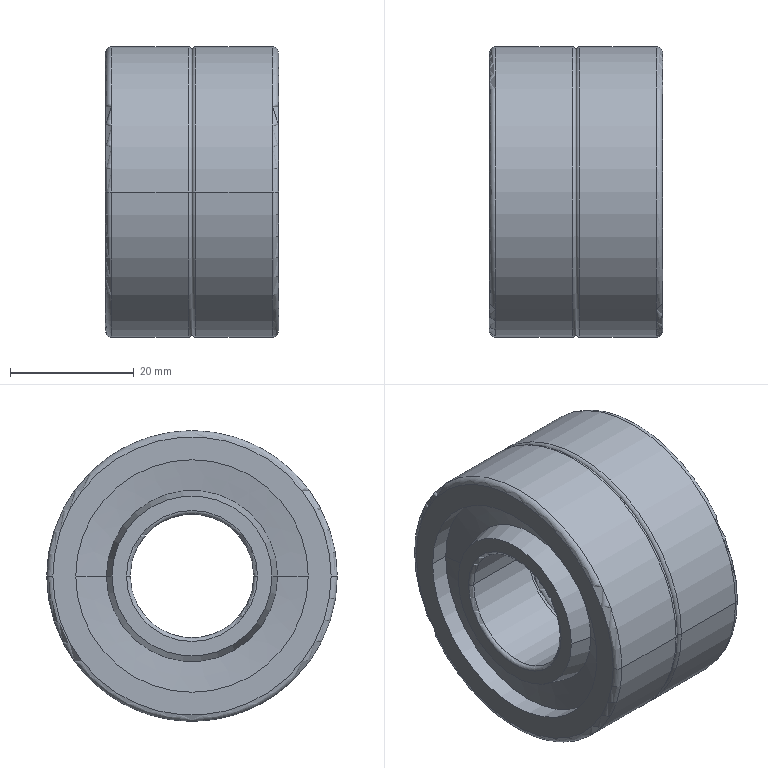Part | NX | 1 solid | 50 faces | box 28 x 47 x 47 mm | volume 32125 mm3 | torus 16 | cone 16 | cylinder 14 | plane 4 | commonest cylinder face diameters 20 x4 37.6 x4 47 x4 29.4 x2
STEP:
#1=CARTESIAN_POINT('',(24.,-11.,0.));
#2=VERTEX_POINT('',#1);
#3=CARTESIAN_POINT('',(23.,-10.,0.));
#4=VERTEX_POINT('',#3);
#5=CARTESIAN_POINT('',(23.,-11.,0.));
#6=DIRECTION('',(0.,0.,-1.));
#7=DIRECTION('',(-1.,0.,0.));
#8=AXIS2_PLACEMENT_3D('',#5,#6,#7);
#9=CIRCLE('',#8,1.);
#10=EDGE_CURVE('',#2,#4,#9,.F.);
#11=ORIENTED_EDGE('',*,*,#10,.T.);
#12=CARTESIAN_POINT('',(23.,10.,0.));
#13=VERTEX_POINT('',#12);
#14=CARTESIAN_POINT('',(23.,0.,0.));
#15=DIRECTION('',(1.,0.,0.));
#16=DIRECTION('',(0.,-1.,0.));
#17=AXIS2_PLACEMENT_3D('',#14,#15,#16);
#18=CIRCLE('',#17,10.);
#19=EDGE_CURVE('',#13,#4,#18,.T.);
#20=ORIENTED_EDGE('',*,*,#19,.F.);
#21=CARTESIAN_POINT('',(24.,11.,0.));
#22=VERTEX_POINT('',#21);
#23=CARTESIAN_POINT('',(23.,11.,0.));
#24=DIRECTION('',(0.,0.,1.));
#25=DIRECTION('',(-1.,0.,0.));
#26=AXIS2_PLACEMENT_3D('',#23,#24,#25);
#27=CIRCLE('',#26,1.);
#28=EDGE_CURVE('',#22,#13,#27,.F.);
#29=ORIENTED_EDGE('',*,*,#28,.F.);
#30=CARTESIAN_POINT('',(24.,0.,0.));
#31=DIRECTION('',(1.,0.,0.));
#32=DIRECTION('',(0.,-1.,0.));
#33=AXIS2_PLACEMENT_3D('',#30,#31,#32);
#34=CIRCLE('',#33,11.);
#35=EDGE_CURVE('',#22,#2,#34,.T.);
#36=ORIENTED_EDGE('',*,*,#35,.T.);
#37=EDGE_LOOP('',(#11,#20,#29,#36));
#38=FACE_BOUND('',#37,.T.);
#39=CARTESIAN_POINT('',(23.,0.,0.));
#40=DIRECTION('',(1.,0.,0.));
#41=DIRECTION('',(0.,-1.,0.));
#42=AXIS2_PLACEMENT_3D('',#39,#40,#41);
#43=TOROIDAL_SURFACE('',#42,11.,1.);
#44=ADVANCED_FACE('',(#38),#43,.T.);
#45=CARTESIAN_POINT('',(38.,-10.6,0.));
#46=VERTEX_POINT('',#45);
#47=CARTESIAN_POINT('',(37.4,-10.,0.));
#48=VERTEX_POINT('',#47);
#49=CARTESIAN_POINT('',(37.4,-10.6,0.));
#50=DIRECTION('',(0.,0.,-1.));
#51=DIRECTION('',(-1.,0.,0.));
#52=AXIS2_PLACEMENT_3D('',#49,#50,#51);
#53=CIRCLE('',#52,0.6);
#54=EDGE_CURVE('',#46,#48,#53,.F.);
#55=ORIENTED_EDGE('',*,*,#54,.T.);
#56=CARTESIAN_POINT('',(37.4,10.,0.));
#57=VERTEX_POINT('',#56);
#58=CARTESIAN_POINT('',(37.4,0.,0.));
#59=DIRECTION('',(1.,0.,0.));
#60=DIRECTION('',(0.,-1.,0.));
#61=AXIS2_PLACEMENT_3D('',#58,#59,#60);
#62=CIRCLE('',#61,10.);
#63=EDGE_CURVE('',#57,#48,#62,.T.);
#64=ORIENTED_EDGE('',*,*,#63,.F.);
#65=CARTESIAN_POINT('',(38.,10.6,0.));
#66=VERTEX_POINT('',#65);
#67=CARTESIAN_POINT('',(37.4,10.6,0.));
#68=DIRECTION('',(0.,0.,1.));
#69=DIRECTION('',(-1.,0.,0.));
#70=AXIS2_PLACEMENT_3D('',#67,#68,#69);
#71=CIRCLE('',#70,0.6);
#72=EDGE_CURVE('',#66,#57,#71,.F.);
#73=ORIENTED_EDGE('',*,*,#72,.F.);
#74=CARTESIAN_POINT('',(38.,0.,0.));
#75=DIRECTION('',(1.,0.,0.));
#76=DIRECTION('',(0.,-1.,0.));
#77=AXIS2_PLACEMENT_3D('',#74,#75,#76);
#78=CIRCLE('',#77,10.6);
#79=EDGE_CURVE('',#66,#46,#78,.T.);
#80=ORIENTED_EDGE('',*,*,#79,.T.);
#81=EDGE_LOOP('',(#55,#64,#73,#80));
#82=FACE_BOUND('',#81,.T.);
#83=CARTESIAN_POINT('',(37.4,0.,0.));
#84=DIRECTION('',(1.,0.,0.));
#85=DIRECTION('',(0.,-1.,0.));
#86=AXIS2_PLACEMENT_3D('',#83,#84,#85);
#87=TOROIDAL_SURFACE('',#86,10.6,0.6);
#88=ADVANCED_FACE('',(#82),#87,.T.);
#89=CARTESIAN_POINT('',(37.,-23.5,0.));
#90=VERTEX_POINT('',#89);
#91=CARTESIAN_POINT('',(37.,23.5,0.));
#92=VERTEX_POINT('',#91);
#93=CARTESIAN_POINT('',(37.,0.,0.));
#94=DIRECTION('',(1.,0.,0.));
#95=DIRECTION('',(0.,-1.,0.));
#96=AXIS2_PLACEMENT_3D('',#93,#94,#95);
#97=CIRCLE('',#96,23.5);
#98=EDGE_CURVE('',#90,#92,#97,.T.);
#99=ORIENTED_EDGE('',*,*,#98,.T.);
#100=CARTESIAN_POINT('',(38.,22.5,0.));
#101=VERTEX_POINT('',#100);
#102=CARTESIAN_POINT('',(37.,22.5,0.));
#103=DIRECTION('',(0.,0.,1.));
#104=DIRECTION('',(-1.,0.,0.));
#105=AXIS2_PLACEMENT_3D('',#102,#103,#104);
#106=CIRCLE('',#105,1.);
#107=EDGE_CURVE('',#101,#92,#106,.T.);
#108=ORIENTED_EDGE('',*,*,#107,.F.);
#109=CARTESIAN_POINT('',(38.,-22.5,0.));
#110=VERTEX_POINT('',#109);
#111=CARTESIAN_POINT('',(38.,0.,0.));
#112=DIRECTION('',(1.,0.,0.));
#113=DIRECTION('',(0.,-1.,0.));
#114=AXIS2_PLACEMENT_3D('',#111,#112,#113);
#115=CIRCLE('',#114,22.5);
#116=EDGE_CURVE('',#110,#101,#115,.T.);
#117=ORIENTED_EDGE('',*,*,#116,.F.);
#118=CARTESIAN_POINT('',(37.,-22.5,0.));
#119=DIRECTION('',(0.,0.,-1.));
#120=DIRECTION('',(-1.,0.,0.));
#121=AXIS2_PLACEMENT_3D('',#118,#119,#120);
#122=CIRCLE('',#121,1.);
#123=EDGE_CURVE('',#110,#90,#122,.T.);
#124=ORIENTED_EDGE('',*,*,#123,.T.);
#125=EDGE_LOOP('',(#99,#108,#117,#124));
#126=FACE_BOUND('',#125,.T.);
#127=CARTESIAN_POINT('',(37.,0.,0.));
#128=DIRECTION('',(1.,0.,0.));
#129=DIRECTION('',(0.,-1.,0.));
#130=AXIS2_PLACEMENT_3D('',#127,#128,#129);
#131=TOROIDAL_SURFACE('',#130,22.5,1.);
#132=ADVANCED_FACE('',(#126),#131,.T.);
#133=CARTESIAN_POINT('',(24.,-22.9,0.));
#134=VERTEX_POINT('',#133);
#135=CARTESIAN_POINT('',(24.,22.9,0.));
#136=VERTEX_POINT('',#135);
#137=CARTESIAN_POINT('',(24.,0.,0.));
#138=DIRECTION('',(1.,0.,0.));
#139=DIRECTION('',(0.,-1.,0.));
#140=AXIS2_PLACEMENT_3D('',#137,#138,#139);
#141=CIRCLE('',#140,22.9);
#142=EDGE_CURVE('',#134,#136,#141,.T.);
#143=ORIENTED_EDGE('',*,*,#142,.F.);
#144=CARTESIAN_POINT('',(23.4,-23.5,0.));
#145=VERTEX_POINT('',#144);
#146=CARTESIAN_POINT('',(23.4,-22.9,0.));
#147=DIRECTION('',(0.,0.,-1.));
#148=DIRECTION('',(-1.,0.,0.));
#149=AXIS2_PLACEMENT_3D('',#146,#147,#148);
#150=CIRCLE('',#149,0.6);
#151=EDGE_CURVE('',#145,#134,#150,.F.);
#152=ORIENTED_EDGE('',*,*,#151,.F.);
#153=CARTESIAN_POINT('',(23.4,23.5,0.));
#154=VERTEX_POINT('',#153);
#155=CARTESIAN_POINT('',(23.4,0.,0.));
#156=DIRECTION('',(1.,0.,0.));
#157=DIRECTION('',(0.,-1.,0.));
#158=AXIS2_PLACEMENT_3D('',#155,#156,#157);
#159=CIRCLE('',#158,23.5);
#160=EDGE_CURVE('',#145,#154,#159,.T.);
#161=ORIENTED_EDGE('',*,*,#160,.T.);
#162=CARTESIAN_POINT('',(23.4,22.9,0.));
#163=DIRECTION('',(0.,0.,1.));
#164=DIRECTION('',(-1.,0.,0.));
#165=AXIS2_PLACEMENT_3D('',#162,#163,#164);
#166=CIRCLE('',#165,0.6);
#167=EDGE_CURVE('',#154,#136,#166,.F.);
#168=ORIENTED_EDGE('',*,*,#167,.T.);
#169=EDGE_LOOP('',(#143,#152,#161,#168));
#170=FACE_BOUND('',#169,.T.);
#171=CARTESIAN_POINT('',(23.4,0.,0.));
#172=DIRECTION('',(1.,0.,0.));
#173=DIRECTION('',(0.,-1.,0.));
#174=AXIS2_PLACEMENT_3D('',#171,#172,#173);
#175=TOROIDAL_SURFACE('',#174,22.9,0.6);
#176=ADVANCED_FACE('',(#170),#175,.T.);
#177=CARTESIAN_POINT('',(24.6,23.5,0.));
#178=VERTEX_POINT('',#177);
#179=CARTESIAN_POINT('',(24.6,-23.5,0.));
#180=VERTEX_POINT('',#179);
#181=CARTESIAN_POINT('',(24.6,0.,0.));
#182=DIRECTION('',(1.,0.,0.));
#183=DIRECTION('',(0.,-1.,0.));
#184=AXIS2_PLACEMENT_3D('',#181,#182,#183);
#185=CIRCLE('',#184,23.5);
#186=EDGE_CURVE('',#178,#180,#185,.T.);
#187=ORIENTED_EDGE('',*,*,#186,.F.);
#188=CARTESIAN_POINT('',(24.6,22.9,0.));
#189=DIRECTION('',(0.,0.,1.));
#190=DIRECTION('',(-1.,0.,0.));
#191=AXIS2_PLACEMENT_3D('',#188,#189,#190);
#192=CIRCLE('',#191,0.6);
#193=EDGE_CURVE('',#178,#136,#192,.T.);
#194=ORIENTED_EDGE('',*,*,#193,.T.);
#195=CARTESIAN_POINT('',(24.,0.,0.));
#196=DIRECTION('',(1.,0.,0.));
#197=DIRECTION('',(0.,-1.,0.));
#198=AXIS2_PLACEMENT_3D('',#195,#196,#197);
#199=CIRCLE('',#198,22.9);
#200=EDGE_CURVE('',#136,#134,#199,.T.);
#201=ORIENTED_EDGE('',*,*,#200,.T.);
#202=CARTESIAN_POINT('',(24.6,-22.9,0.));
#203=DIRECTION('',(0.,0.,-1.));
#204=DIRECTION('',(-1.,0.,0.));
#205=AXIS2_PLACEMENT_3D('',#202,#203,#204);
#206=CIRCLE('',#205,0.6);
#207=EDGE_CURVE('',#180,#134,#206,.T.);
#208=ORIENTED_EDGE('',*,*,#207,.F.);
#209=EDGE_LOOP('',(#187,#194,#201,#208));
#210=FACE_BOUND('',#209,.T.);
#211=CARTESIAN_POINT('',(24.6,0.,0.));
#212=DIRECTION('',(1.,0.,0.));
#213=DIRECTION('',(0.,-1.,0.));
#214=AXIS2_PLACEMENT_3D('',#211,#212,#213);
#215=TOROIDAL_SURFACE('',#214,22.9,0.6);
#216=ADVANCED_FACE('',(#210),#215,.T.);
#217=CARTESIAN_POINT('',(10.,22.5,0.));
#218=VERTEX_POINT('',#217);
#219=CARTESIAN_POINT('',(10.,-22.5,0.));
#220=VERTEX_POINT('',#219);
#221=CARTESIAN_POINT('',(10.,0.,0.));
#222=DIRECTION('',(1.,0.,0.));
#223=DIRECTION('',(0.,-1.,0.));
#224=AXIS2_PLACEMENT_3D('',#221,#222,#223);
#225=CIRCLE('',#224,22.5);
#226=EDGE_CURVE('',#218,#220,#225,.T.);
#227=ORIENTED_EDGE('',*,*,#226,.T.);
#228=CARTESIAN_POINT('',(11.,-23.5,0.));
#229=VERTEX_POINT('',#228);
#230=CARTESIAN_POINT('',(11.,-22.5,0.));
#231=DIRECTION('',(0.,0.,-1.));
#232=DIRECTION('',(-1.,0.,0.));
#233=AXIS2_PLACEMENT_3D('',#230,#231,#232);
#234=CIRCLE('',#233,1.);
#235=EDGE_CURVE('',#220,#229,#234,.F.);
#236=ORIENTED_EDGE('',*,*,#235,.T.);
#237=CARTESIAN_POINT('',(11.,23.5,0.));
#238=VERTEX_POINT('',#237);
#239=CARTESIAN_POINT('',(11.,0.,0.));
#240=DIRECTION('',(1.,0.,0.));
#241=DIRECTION('',(0.,-1.,0.));
#242=AXIS2_PLACEMENT_3D('',#239,#240,#241);
#243=CIRCLE('',#242,23.5);
#244=EDGE_CURVE('',#238,#229,#243,.T.);
#245=ORIENTED_EDGE('',*,*,#244,.F.);
#246=CARTESIAN_POINT('',(11.,22.5,0.));
#247=DIRECTION('',(0.,0.,1.));
#248=DIRECTION('',(-1.,0.,0.));
#249=AXIS2_PLACEMENT_3D('',#246,#247,#248);
#250=CIRCLE('',#249,1.);
#251=EDGE_CURVE('',#218,#238,#250,.F.);
#252=ORIENTED_EDGE('',*,*,#251,.F.);
#253=EDGE_LOOP('',(#227,#236,#245,#252));
#254=FACE_BOUND('',#253,.T.);
#255=CARTESIAN_POINT('',(11.,0.,0.));
#256=DIRECTION('',(1.,0.,0.));
#257=DIRECTION('',(0.,-1.,0.));
#258=AXIS2_PLACEMENT_3D('',#255,#256,#257);
#259=TOROIDAL_SURFACE('',#258,22.5,1.);
#260=ADVANCED_FACE('',(#254),#259,.T.);
#261=CARTESIAN_POINT('',(10.,-10.6,0.));
#262=VERTEX_POINT('',#261);
#263=CARTESIAN_POINT('',(10.,10.6,0.));
#264=VERTEX_POINT('',#263);
#265=CARTESIAN_POINT('',(10.,0.,0.));
#266=DIRECTION('',(1.,0.,0.));
#267=DIRECTION('',(0.,-1.,0.));
#268=AXIS2_PLACEMENT_3D('',#265,#266,#267);
#269=CIRCLE('',#268,10.6);
#270=EDGE_CURVE('',#262,#264,#269,.T.);
#271=ORIENTED_EDGE('',*,*,#270,.F.);
#272=CARTESIAN_POINT('',(10.6,-10.,0.));
#273=VERTEX_POINT('',#272);
#274=CARTESIAN_POINT('',(10.6,-10.6,0.));
#275=DIRECTION('',(0.,0.,-1.));
#276=DIRECTION('',(-1.,0.,0.));
#277=AXIS2_PLACEMENT_3D('',#274,#275,#276);
#278=CIRCLE('',#277,0.6);
#279=EDGE_CURVE('',#273,#262,#278,.F.);
#280=ORIENTED_EDGE('',*,*,#279,.F.);
#281=CARTESIAN_POINT('',(10.6,10.,0.));
#282=VERTEX_POINT('',#281);
#283=CARTESIAN_POINT('',(10.6,0.,0.));
#284=DIRECTION('',(1.,0.,0.));
#285=DIRECTION('',(0.,-1.,0.));
#286=AXIS2_PLACEMENT_3D('',#283,#284,#285);
#287=CIRCLE('',#286,10.);
#288=EDGE_CURVE('',#273,#282,#287,.T.);
#289=ORIENTED_EDGE('',*,*,#288,.T.);
#290=CARTESIAN_POINT('',(10.6,10.6,0.));
#291=DIRECTION('',(0.,0.,1.));
#292=DIRECTION('',(-1.,0.,0.));
#293=AXIS2_PLACEMENT_3D('',#290,#291,#292);
#294=CIRCLE('',#293,0.6);
#295=EDGE_CURVE('',#282,#264,#294,.F.);
#296=ORIENTED_EDGE('',*,*,#295,.T.);
#297=EDGE_LOOP('',(#271,#280,#289,#296));
#298=FACE_BOUND('',#297,.T.);
#299=CARTESIAN_POINT('',(10.6,0.,0.));
#300=DIRECTION('',(1.,0.,0.));
#301=DIRECTION('',(0.,-1.,0.));
#302=AXIS2_PLACEMENT_3D('',#299,#300,#301);
#303=TOROIDAL_SURFACE('',#302,10.6,0.6);
#304=ADVANCED_FACE('',(#298),#303,.T.);
#305=CARTESIAN_POINT('',(25.,10.,0.));
#306=VERTEX_POINT('',#305);
#307=CARTESIAN_POINT('',(25.,-10.,0.));
#308=VERTEX_POINT('',#307);
#309=CARTESIAN_POINT('',(25.,0.,0.));
#310=DIRECTION('',(1.,0.,0.));
#311=DIRECTION('',(0.,-1.,0.));
#312=AXIS2_PLACEMENT_3D('',#309,#310,#311);
#313=CIRCLE('',#312,10.);
#314=EDGE_CURVE('',#306,#308,#313,.T.);
#315=ORIENTED_EDGE('',*,*,#314,.T.);
#316=CARTESIAN_POINT('',(25.,-11.,0.));
#317=DIRECTION('',(0.,0.,-1.));
#318=DIRECTION('',(-1.,0.,0.));
#319=AXIS2_PLACEMENT_3D('',#316,#317,#318);
#320=CIRCLE('',#319,1.);
#321=EDGE_CURVE('',#308,#2,#320,.F.);
#322=ORIENTED_EDGE('',*,*,#321,.T.);
#323=ORIENTED_EDGE('',*,*,#35,.F.);
#324=CARTESIAN_POINT('',(25.,11.,0.));
#325=DIRECTION('',(0.,0.,1.));
#326=DIRECTION('',(-1.,0.,0.));
#327=AXIS2_PLACEMENT_3D('',#324,#325,#326);
#328=CIRCLE('',#327,1.);
#329=EDGE_CURVE('',#306,#22,#328,.F.);
#330=ORIENTED_EDGE('',*,*,#329,.F.);
#331=EDGE_LOOP('',(#315,#322,#323,#330));
#332=FACE_BOUND('',#331,.T.);
#333=CARTESIAN_POINT('',(25.,0.,0.));
#334=DIRECTION('',(1.,0.,0.));
#335=DIRECTION('',(0.,-1.,0.));
#336=AXIS2_PLACEMENT_3D('',#333,#334,#335);
#337=TOROIDAL_SURFACE('',#336,11.,1.);
#338=ADVANCED_FACE('',(#332),#337,.T.);
#339=CARTESIAN_POINT('',(34.43,13.836,0.));
#340=VERTEX_POINT('',#339);
#341=CARTESIAN_POINT('',(34.43,-13.836,0.));
#342=VERTEX_POINT('',#341);
#343=CARTESIAN_POINT('',(34.43,0.,0.));
#344=DIRECTION('',(1.,0.,0.));
#345=DIRECTION('',(0.,-1.,0.));
#346=AXIS2_PLACEMENT_3D('',#343,#344,#345);
#347=CIRCLE('',#346,13.836);
#348=EDGE_CURVE('',#340,#342,#347,.T.);
#349=ORIENTED_EDGE('',*,*,#348,.F.);
#350=CARTESIAN_POINT('',(35.006,18.8,0.));
#351=VERTEX_POINT('',#350);
#352=CARTESIAN_POINT('',(34.718,16.318,0.));
#353=DIRECTION('',(0.1154,0.9933,0.));
#354=VECTOR('',#353,1000.);
#355=LINE('',#352,#354);
#356=EDGE_CURVE('',#340,#351,#355,.T.);
#357=ORIENTED_EDGE('',*,*,#356,.T.);
#358=CARTESIAN_POINT('',(35.006,-18.8,0.));
#359=VERTEX_POINT('',#358);
#360=CARTESIAN_POINT('',(35.006,0.,0.));
#361=DIRECTION('',(1.,0.,0.));
#362=DIRECTION('',(0.,-1.,0.));
#363=AXIS2_PLACEMENT_3D('',#360,#361,#362);
#364=CIRCLE('',#363,18.8);
#365=EDGE_CURVE('',#351,#359,#364,.T.);
#366=ORIENTED_EDGE('',*,*,#365,.T.);
#367=CARTESIAN_POINT('',(34.718,-16.318,0.));
#368=DIRECTION('',(0.1154,-0.9933,0.));
#369=VECTOR('',#368,1000.);
#370=LINE('',#367,#369);
#371=EDGE_CURVE('',#342,#359,#370,.T.);
#372=ORIENTED_EDGE('',*,*,#371,.F.);
#373=EDGE_LOOP('',(#349,#357,#366,#372));
#374=FACE_BOUND('',#373,.T.);
#375=CARTESIAN_POINT('',(34.718,0.,0.));
#376=DIRECTION('',(1.,0.,0.));
#377=DIRECTION('',(0.,-1.,0.));
#378=AXIS2_PLACEMENT_3D('',#375,#376,#377);
#379=CONICAL_SURFACE('',#378,16.318,1.455);
#380=ADVANCED_FACE('',(#374),#379,.F.);
#381=CARTESIAN_POINT('',(13.57,-13.836,0.));
#382=VERTEX_POINT('',#381);
#383=CARTESIAN_POINT('',(10.,-12.938,0.));
#384=VERTEX_POINT('',#383);
#385=CARTESIAN_POINT('',(11.785,-13.387,0.));
#386=DIRECTION('',(0.9697,-0.2442,0.));
#387=VECTOR('',#386,1000.);
#388=LINE('',#385,#387);
#389=EDGE_CURVE('',#382,#384,#388,.F.);
#390=ORIENTED_EDGE('',*,*,#389,.T.);
#391=CARTESIAN_POINT('',(10.,12.938,0.));
#392=VERTEX_POINT('',#391);
#393=CARTESIAN_POINT('',(10.,0.,0.));
#394=DIRECTION('',(1.,0.,0.));
#395=DIRECTION('',(0.,-1.,0.));
#396=AXIS2_PLACEMENT_3D('',#393,#394,#395);
#397=CIRCLE('',#396,12.938);
#398=EDGE_CURVE('',#384,#392,#397,.T.);
#399=ORIENTED_EDGE('',*,*,#398,.T.);
#400=CARTESIAN_POINT('',(13.57,13.836,0.));
#401=VERTEX_POINT('',#400);
#402=CARTESIAN_POINT('',(11.785,13.387,0.));
#403=DIRECTION('',(0.9697,0.2442,0.));
#404=VECTOR('',#403,1000.);
#405=LINE('',#402,#404);
#406=EDGE_CURVE('',#401,#392,#405,.F.);
#407=ORIENTED_EDGE('',*,*,#406,.F.);
#408=CARTESIAN_POINT('',(13.57,0.,0.));
#409=DIRECTION('',(1.,0.,0.));
#410=DIRECTION('',(0.,-1.,0.));
#411=AXIS2_PLACEMENT_3D('',#408,#409,#410);
#412=CIRCLE('',#411,13.836);
#413=EDGE_CURVE('',#382,#401,#412,.T.);
#414=ORIENTED_EDGE('',*,*,#413,.F.);
#415=EDGE_LOOP('',(#390,#399,#407,#414));
#416=FACE_BOUND('',#415,.T.);
#417=CARTESIAN_POINT('',(11.785,0.,0.));
#418=DIRECTION('',(1.,0.,0.));
#419=DIRECTION('',(0.,-1.,0.));
#420=AXIS2_PLACEMENT_3D('',#417,#418,#419);
#421=CONICAL_SURFACE('',#420,13.387,0.2467);
#422=ADVANCED_FACE('',(#416),#421,.T.);
#423=CARTESIAN_POINT('',(10.6,0.,0.));
#424=DIRECTION('',(1.,0.,0.));
#425=DIRECTION('',(0.,-1.,0.));
#426=AXIS2_PLACEMENT_3D('',#423,#424,#425);
#427=CIRCLE('',#426,10.);
#428=EDGE_CURVE('',#282,#273,#427,.T.);
#429=ORIENTED_EDGE('',*,*,#428,.F.);
#430=CARTESIAN_POINT('',(16.8,10.,0.));
#431=DIRECTION('',(-1.,0.,0.));
#432=VECTOR('',#431,1000.);
#433=LINE('',#430,#432);
#434=EDGE_CURVE('',#13,#282,#433,.T.);
#435=ORIENTED_EDGE('',*,*,#434,.F.);
#436=ORIENTED_EDGE('',*,*,#19,.T.);
#437=CARTESIAN_POINT('',(16.8,-10.,0.));
#438=DIRECTION('',(-1.,0.,0.));
#439=VECTOR('',#438,1000.);
#440=LINE('',#437,#439);
#441=EDGE_CURVE('',#4,#273,#440,.T.);
#442=ORIENTED_EDGE('',*,*,#441,.T.);
#443=EDGE_LOOP('',(#429,#435,#436,#442));
#444=FACE_BOUND('',#443,.T.);
#445=CARTESIAN_POINT('',(16.8,0.,0.));
#446=DIRECTION('',(-1.,0.,0.));
#447=DIRECTION('',(0.,-1.,0.));
#448=AXIS2_PLACEMENT_3D('',#445,#446,#447);
#449=CYLINDRICAL_SURFACE('',#448,10.);
#450=ADVANCED_FACE('',(#444),#449,.F.);
#451=ORIENTED_EDGE('',*,*,#314,.F.);
#452=CARTESIAN_POINT('',(31.2,10.,0.));
#453=DIRECTION('',(-1.,0.,0.));
#454=VECTOR('',#453,1000.);
#455=LINE('',#452,#454);
#456=EDGE_CURVE('',#57,#306,#455,.T.);
#457=ORIENTED_EDGE('',*,*,#456,.F.);
#458=ORIENTED_EDGE('',*,*,#63,.T.);
#459=CARTESIAN_POINT('',(31.2,-10.,0.));
#460=DIRECTION('',(-1.,0.,0.));
#461=VECTOR('',#460,1000.);
#462=LINE('',#459,#461);
#463=EDGE_CURVE('',#48,#308,#462,.T.);
#464=ORIENTED_EDGE('',*,*,#463,.T.);
#465=EDGE_LOOP('',(#451,#457,#458,#464));
#466=FACE_BOUND('',#465,.T.);
#467=CARTESIAN_POINT('',(31.2,0.,0.));
#468=DIRECTION('',(-1.,0.,0.));
#469=DIRECTION('',(0.,-1.,0.));
#470=AXIS2_PLACEMENT_3D('',#467,#468,#469);
#471=CYLINDRICAL_SURFACE('',#470,10.);
#472=ADVANCED_FACE('',(#466),#471,.F.);
#473=CARTESIAN_POINT('',(38.,12.938,0.));
#474=VERTEX_POINT('',#473);
#475=CARTESIAN_POINT('',(36.215,13.387,0.));
#476=DIRECTION('',(-0.9697,0.2442,0.));
#477=VECTOR('',#476,1000.);
#478=LINE('',#475,#477);
#479=EDGE_CURVE('',#474,#340,#478,.T.);
#480=ORIENTED_EDGE('',*,*,#479,.F.);
#481=CARTESIAN_POINT('',(38.,-12.938,0.));
#482=VERTEX_POINT('',#481);
#483=CARTESIAN_POINT('',(38.,0.,0.));
#484=DIRECTION('',(1.,0.,0.));
#485=DIRECTION('',(0.,-1.,0.));
#486=AXIS2_PLACEMENT_3D('',#483,#484,#485);
#487=CIRCLE('',#486,12.938);
#488=EDGE_CURVE('',#482,#474,#487,.T.);
#489=ORIENTED_EDGE('',*,*,#488,.F.);
#490=CARTESIAN_POINT('',(36.215,-13.387,0.));
#491=DIRECTION('',(-0.9697,-0.2442,0.));
#492=VECTOR('',#491,1000.);
#493=LINE('',#490,#492);
#494=EDGE_CURVE('',#482,#342,#493,.T.);
#495=ORIENTED_EDGE('',*,*,#494,.T.);
#496=CARTESIAN_POINT('',(34.43,0.,0.));
#497=DIRECTION('',(1.,0.,0.));
#498=DIRECTION('',(0.,-1.,0.));
#499=AXIS2_PLACEMENT_3D('',#496,#497,#498);
#500=CIRCLE('',#499,13.836);
#501=EDGE_CURVE('',#342,#340,#500,.T.);
#502=ORIENTED_EDGE('',*,*,#501,.T.);
#503=EDGE_LOOP('',(#480,#489,#495,#502));
#504=FACE_BOUND('',#503,.T.);
#505=CARTESIAN_POINT('',(36.215,0.,0.));
#506=DIRECTION('',(-1.,0.,0.));
#507=DIRECTION('',(0.,1.,0.));
#508=AXIS2_PLACEMENT_3D('',#505,#506,#507);
#509=CONICAL_SURFACE('',#508,13.387,0.2467);
#510=ADVANCED_FACE('',(#504),#509,.T.);
#511=CARTESIAN_POINT('',(12.994,-18.8,0.));
#512=VERTEX_POINT('',#511);
#513=CARTESIAN_POINT('',(12.994,18.8,0.));
#514=VERTEX_POINT('',#513);
#515=CARTESIAN_POINT('',(12.994,0.,0.));
#516=DIRECTION('',(1.,0.,0.));
#517=DIRECTION('',(0.,-1.,0.));
#518=AXIS2_PLACEMENT_3D('',#515,#516,#517);
#519=CIRCLE('',#518,18.8);
#520=EDGE_CURVE('',#512,#514,#519,.T.);
#521=ORIENTED_EDGE('',*,*,#520,.F.);
#522=CARTESIAN_POINT('',(13.282,-16.318,0.));
#523=DIRECTION('',(-0.1154,-0.9933,0.));
#524=VECTOR('',#523,1000.);
#525=LINE('',#522,#524);
#526=EDGE_CURVE('',#512,#382,#525,.F.);
#527=ORIENTED_EDGE('',*,*,#526,.T.);
#528=ORIENTED_EDGE('',*,*,#413,.T.);
#529=CARTESIAN_POINT('',(13.282,16.318,0.));
#530=DIRECTION('',(-0.1154,0.9933,0.));
#531=VECTOR('',#530,1000.);
#532=LINE('',#529,#531);
#533=EDGE_CURVE('',#514,#401,#532,.F.);
#534=ORIENTED_EDGE('',*,*,#533,.F.);
#535=EDGE_LOOP('',(#521,#527,#528,#534));
#536=FACE_BOUND('',#535,.T.);
#537=CARTESIAN_POINT('',(13.282,0.,0.));
#538=DIRECTION('',(-1.,0.,0.));
#539=DIRECTION('',(0.,1.,0.));
#540=AXIS2_PLACEMENT_3D('',#537,#538,#539);
#541=CONICAL_SURFACE('',#540,16.318,1.455);
#542=ADVANCED_FACE('',(#536),#541,.F.);
#543=CARTESIAN_POINT('',(38.,-18.8,0.));
#544=VERTEX_POINT('',#543);
#545=CARTESIAN_POINT('',(36.503,-18.8,0.));
#546=DIRECTION('',(-1.,0.,0.));
#547=VECTOR('',#546,1000.);
#548=LINE('',#545,#547);
#549=EDGE_CURVE('',#544,#359,#548,.T.);
#550=ORIENTED_EDGE('',*,*,#549,.T.);
#551=ORIENTED_EDGE('',*,*,#365,.F.);
#552=CARTESIAN_POINT('',(38.,18.8,0.));
#553=VERTEX_POINT('',#552);
#554=CARTESIAN_POINT('',(36.503,18.8,0.));
#555=DIRECTION('',(-1.,0.,0.));
#556=VECTOR('',#555,1000.);
#557=LINE('',#554,#556);
#558=EDGE_CURVE('',#553,#351,#557,.T.);
#559=ORIENTED_EDGE('',*,*,#558,.F.);
#560=CARTESIAN_POINT('',(38.,0.,0.));
#561=DIRECTION('',(1.,0.,0.));
#562=DIRECTION('',(0.,-1.,0.));
#563=AXIS2_PLACEMENT_3D('',#560,#561,#562);
#564=CIRCLE('',#563,18.8);
#565=EDGE_CURVE('',#553,#544,#564,.T.);
#566=ORIENTED_EDGE('',*,*,#565,.T.);
#567=EDGE_LOOP('',(#550,#551,#559,#566));
#568=FACE_BOUND('',#567,.T.);
#569=CARTESIAN_POINT('',(36.503,0.,0.));
#570=DIRECTION('',(-1.,0.,0.));
#571=DIRECTION('',(0.,-1.,0.));
#572=AXIS2_PLACEMENT_3D('',#569,#570,#571);
#573=CYLINDRICAL_SURFACE('',#572,18.8);
#574=ADVANCED_FACE('',(#568),#573,.F.);
#575=ORIENTED_EDGE('',*,*,#186,.T.);
#576=CARTESIAN_POINT('',(30.8,-23.5,0.));
#577=DIRECTION('',(-1.,0.,0.));
#578=VECTOR('',#577,1000.);
#579=LINE('',#576,#578);
#580=EDGE_CURVE('',#180,#90,#579,.F.);
#581=ORIENTED_EDGE('',*,*,#580,.T.);
#582=CARTESIAN_POINT('',(37.,0.,0.));
#583=DIRECTION('',(1.,0.,0.));
#584=DIRECTION('',(0.,-1.,0.));
#585=AXIS2_PLACEMENT_3D('',#582,#583,#584);
#586=CIRCLE('',#585,23.5);
#587=EDGE_CURVE('',#92,#90,#586,.T.);
#588=ORIENTED_EDGE('',*,*,#587,.F.);
#589=CARTESIAN_POINT('',(30.8,23.5,0.));
#590=DIRECTION('',(-1.,0.,0.));
#591=VECTOR('',#590,1000.);
#592=LINE('',#589,#591);
#593=EDGE_CURVE('',#178,#92,#592,.F.);
#594=ORIENTED_EDGE('',*,*,#593,.F.);
#595=EDGE_LOOP('',(#575,#581,#588,#594));
#596=FACE_BOUND('',#595,.T.);
#597=CARTESIAN_POINT('',(30.8,0.,0.));
#598=DIRECTION('',(-1.,0.,0.));
#599=DIRECTION('',(0.,-1.,0.));
#600=AXIS2_PLACEMENT_3D('',#597,#598,#599);
#601=CYLINDRICAL_SURFACE('',#600,23.5);
#602=ADVANCED_FACE('',(#596),#601,.T.);
#603=CARTESIAN_POINT('',(11.,0.,0.));
#604=DIRECTION('',(1.,0.,0.));
#605=DIRECTION('',(0.,-1.,0.));
#606=AXIS2_PLACEMENT_3D('',#603,#604,#605);
#607=CIRCLE('',#606,23.5);
#608=EDGE_CURVE('',#229,#238,#607,.T.);
#609=ORIENTED_EDGE('',*,*,#608,.T.);
#610=CARTESIAN_POINT('',(17.2,23.5,0.));
#611=DIRECTION('',(-1.,0.,0.));
#612=VECTOR('',#611,1000.);
#613=LINE('',#610,#612);
#614=EDGE_CURVE('',#154,#238,#613,.T.);
#615=ORIENTED_EDGE('',*,*,#614,.F.);
#616=ORIENTED_EDGE('',*,*,#160,.F.);
#617=CARTESIAN_POINT('',(17.2,-23.5,0.));
#618=DIRECTION('',(-1.,0.,0.));
#619=VECTOR('',#618,1000.);
#620=LINE('',#617,#619);
#621=EDGE_CURVE('',#145,#229,#620,.T.);
#622=ORIENTED_EDGE('',*,*,#621,.T.);
#623=EDGE_LOOP('',(#609,#615,#616,#622));
#624=FACE_BOUND('',#623,.T.);
#625=CARTESIAN_POINT('',(17.2,0.,0.));
#626=DIRECTION('',(-1.,0.,0.));
#627=DIRECTION('',(0.,-1.,0.));
#628=AXIS2_PLACEMENT_3D('',#625,#626,#627);
#629=CYLINDRICAL_SURFACE('',#628,23.5);
#630=ADVANCED_FACE('',(#624),#629,.T.);
#631=CARTESIAN_POINT('',(10.,-18.8,0.));
#632=VERTEX_POINT('',#631);
#633=CARTESIAN_POINT('',(11.497,-18.8,0.));
#634=DIRECTION('',(-1.,0.,0.));
#635=VECTOR('',#634,1000.);
#636=LINE('',#633,#635);
#637=EDGE_CURVE('',#632,#512,#636,.F.);
#638=ORIENTED_EDGE('',*,*,#637,.F.);
#639=CARTESIAN_POINT('',(10.,18.8,0.));
#640=VERTEX_POINT('',#639);
#641=CARTESIAN_POINT('',(10.,0.,0.));
#642=DIRECTION('',(1.,0.,0.));
#643=DIRECTION('',(0.,-1.,0.));
#644=AXIS2_PLACEMENT_3D('',#641,#642,#643);
#645=CIRCLE('',#644,18.8);
#646=EDGE_CURVE('',#640,#632,#645,.T.);
#647=ORIENTED_EDGE('',*,*,#646,.F.);
#648=CARTESIAN_POINT('',(11.497,18.8,0.));
#649=DIRECTION('',(-1.,0.,0.));
#650=VECTOR('',#649,1000.);
#651=LINE('',#648,#650);
#652=EDGE_CURVE('',#640,#514,#651,.F.);
#653=ORIENTED_EDGE('',*,*,#652,.T.);
#654=CARTESIAN_POINT('',(12.994,0.,0.));
#655=DIRECTION('',(1.,0.,0.));
#656=DIRECTION('',(0.,-1.,0.));
#657=AXIS2_PLACEMENT_3D('',#654,#655,#656);
#658=CIRCLE('',#657,18.8);
#659=EDGE_CURVE('',#514,#512,#658,.T.);
#660=ORIENTED_EDGE('',*,*,#659,.T.);
#661=EDGE_LOOP('',(#638,#647,#653,#660));
#662=FACE_BOUND('',#661,.T.);
#663=CARTESIAN_POINT('',(11.497,0.,0.));
#664=DIRECTION('',(-1.,0.,0.));
#665=DIRECTION('',(0.,-1.,0.));
#666=AXIS2_PLACEMENT_3D('',#663,#664,#665);
#667=CYLINDRICAL_SURFACE('',#666,18.8);
#668=ADVANCED_FACE('',(#662),#667,.F.);
#669=ORIENTED_EDGE('',*,*,#270,.T.);
#670=CARTESIAN_POINT('',(10.,0.,0.));
#671=DIRECTION('',(1.,0.,0.));
#672=DIRECTION('',(0.,-1.,0.));
#673=AXIS2_PLACEMENT_3D('',#670,#671,#672);
#674=CIRCLE('',#673,10.6);
#675=EDGE_CURVE('',#264,#262,#674,.T.);
#676=ORIENTED_EDGE('',*,*,#675,.T.);
#677=EDGE_LOOP('',(#669,#676));
#678=FACE_BOUND('',#677,.T.);
#679=CARTESIAN_POINT('',(10.,0.,0.));
#680=DIRECTION('',(1.,0.,0.));
#681=DIRECTION('',(0.,-1.,0.));
#682=AXIS2_PLACEMENT_3D('',#679,#680,#681);
#683=CIRCLE('',#682,12.938);
#684=EDGE_CURVE('',#392,#384,#683,.T.);
#685=ORIENTED_EDGE('',*,*,#684,.F.);
#686=ORIENTED_EDGE('',*,*,#398,.F.);
#687=EDGE_LOOP('',(#685,#686));
#688=FACE_BOUND('',#687,.T.);
#689=CARTESIAN_POINT('',(10.,-11.769,0.));
#690=DIRECTION('',(-1.,0.,0.));
#691=DIRECTION('',(0.,0.,1.));
#692=AXIS2_PLACEMENT_3D('',#689,#690,#691);
#693=PLANE('',#692);
#694=ADVANCED_FACE('',(#678,#688),#693,.T.);
#695=CARTESIAN_POINT('',(38.,0.,0.));
#696=DIRECTION('',(1.,0.,0.));
#697=DIRECTION('',(0.,-1.,0.));
#698=AXIS2_PLACEMENT_3D('',#695,#696,#697);
#699=CIRCLE('',#698,10.6);
#700=EDGE_CURVE('',#46,#66,#699,.T.);
#701=ORIENTED_EDGE('',*,*,#700,.F.);
#702=ORIENTED_EDGE('',*,*,#79,.F.);
#703=EDGE_LOOP('',(#701,#702));
#704=FACE_BOUND('',#703,.T.);
#705=CARTESIAN_POINT('',(38.,0.,0.));
#706=DIRECTION('',(1.,0.,0.));
#707=DIRECTION('',(0.,-1.,0.));
#708=AXIS2_PLACEMENT_3D('',#705,#706,#707);
#709=CIRCLE('',#708,12.938);
#710=EDGE_CURVE('',#474,#482,#709,.T.);
#711=ORIENTED_EDGE('',*,*,#710,.T.);
#712=ORIENTED_EDGE('',*,*,#488,.T.);
#713=EDGE_LOOP('',(#711,#712));
#714=FACE_BOUND('',#713,.T.);
#715=CARTESIAN_POINT('',(38.,-11.769,0.));
#716=DIRECTION('',(1.,0.,0.));
#717=DIRECTION('',(0.,1.,0.));
#718=AXIS2_PLACEMENT_3D('',#715,#716,#717);
#719=PLANE('',#718);
#720=ADVANCED_FACE('',(#704,#714),#719,.T.);
#721=CARTESIAN_POINT('',(10.,0.,0.));
#722=DIRECTION('',(1.,0.,0.));
#723=DIRECTION('',(0.,-1.,0.));
#724=AXIS2_PLACEMENT_3D('',#721,#722,#723);
#725=CIRCLE('',#724,18.8);
#726=EDGE_CURVE('',#632,#640,#725,.T.);
#727=ORIENTED_EDGE('',*,*,#726,.T.);
#728=ORIENTED_EDGE('',*,*,#646,.T.);
#729=EDGE_LOOP('',(#727,#728));
#730=FACE_BOUND('',#729,.T.);
#731=ORIENTED_EDGE('',*,*,#226,.F.);
#732=CARTESIAN_POINT('',(10.,0.,0.));
#733=DIRECTION('',(1.,0.,0.));
#734=DIRECTION('',(0.,-1.,0.));
#735=AXIS2_PLACEMENT_3D('',#732,#733,#734);
#736=CIRCLE('',#735,22.5);
#737=EDGE_CURVE('',#220,#218,#736,.T.);
#738=ORIENTED_EDGE('',*,*,#737,.F.);
#739=EDGE_LOOP('',(#731,#738));
#740=FACE_BOUND('',#739,.T.);
#741=CARTESIAN_POINT('',(10.,-20.65,0.));
#742=DIRECTION('',(-1.,0.,0.));
#743=DIRECTION('',(0.,0.,1.));
#744=AXIS2_PLACEMENT_3D('',#741,#742,#743);
#745=PLANE('',#744);
#746=ADVANCED_FACE('',(#730,#740),#745,.T.);
#747=CARTESIAN_POINT('',(38.,0.,0.));
#748=DIRECTION('',(1.,0.,0.));
#749=DIRECTION('',(0.,-1.,0.));
#750=AXIS2_PLACEMENT_3D('',#747,#748,#749);
#751=CIRCLE('',#750,18.8);
#752=EDGE_CURVE('',#544,#553,#751,.T.);
#753=ORIENTED_EDGE('',*,*,#752,.F.);
#754=ORIENTED_EDGE('',*,*,#565,.F.);
#755=EDGE_LOOP('',(#753,#754));
#756=FACE_BOUND('',#755,.T.);
#757=CARTESIAN_POINT('',(38.,0.,0.));
#758=DIRECTION('',(1.,0.,0.));
#759=DIRECTION('',(0.,-1.,0.));
#760=AXIS2_PLACEMENT_3D('',#757,#758,#759);
#761=CIRCLE('',#760,22.5);
#762=EDGE_CURVE('',#101,#110,#761,.T.);
#763=ORIENTED_EDGE('',*,*,#762,.T.);
#764=ORIENTED_EDGE('',*,*,#116,.T.);
#765=EDGE_LOOP('',(#763,#764));
#766=FACE_BOUND('',#765,.T.);
#767=CARTESIAN_POINT('',(38.,-20.65,0.));
#768=DIRECTION('',(1.,0.,0.));
#769=DIRECTION('',(0.,1.,0.));
#770=AXIS2_PLACEMENT_3D('',#767,#768,#769);
#771=PLANE('',#770);
#772=ADVANCED_FACE('',(#756,#766),#771,.T.);
#773=ORIENTED_EDGE('',*,*,#762,.F.);
#774=ORIENTED_EDGE('',*,*,#107,.T.);
#775=ORIENTED_EDGE('',*,*,#587,.T.);
#776=ORIENTED_EDGE('',*,*,#123,.F.);
#777=EDGE_LOOP('',(#773,#774,#775,#776));
#778=FACE_BOUND('',#777,.T.);
#779=CARTESIAN_POINT('',(37.,0.,0.));
#780=DIRECTION('',(1.,0.,0.));
#781=DIRECTION('',(0.,-1.,0.));
#782=AXIS2_PLACEMENT_3D('',#779,#780,#781);
#783=TOROIDAL_SURFACE('',#782,22.5,1.);
#784=ADVANCED_FACE('',(#778),#783,.T.);
#785=ORIENTED_EDGE('',*,*,#98,.F.);
#786=ORIENTED_EDGE('',*,*,#580,.F.);
#787=CARTESIAN_POINT('',(24.6,0.,0.));
#788=DIRECTION('',(1.,0.,0.));
#789=DIRECTION('',(0.,-1.,0.));
#790=AXIS2_PLACEMENT_3D('',#787,#788,#789);
#791=CIRCLE('',#790,23.5);
#792=EDGE_CURVE('',#180,#178,#791,.T.);
#793=ORIENTED_EDGE('',*,*,#792,.T.);
#794=ORIENTED_EDGE('',*,*,#593,.T.);
#795=EDGE_LOOP('',(#785,#786,#793,#794));
#796=FACE_BOUND('',#795,.T.);
#797=CARTESIAN_POINT('',(30.8,0.,0.));
#798=DIRECTION('',(-1.,0.,0.));
#799=DIRECTION('',(0.,-1.,0.));
#800=AXIS2_PLACEMENT_3D('',#797,#798,#799);
#801=CYLINDRICAL_SURFACE('',#800,23.5);
#802=ADVANCED_FACE('',(#796),#801,.T.);
#803=ORIENTED_EDGE('',*,*,#142,.T.);
#804=ORIENTED_EDGE('',*,*,#193,.F.);
#805=ORIENTED_EDGE('',*,*,#792,.F.);
#806=ORIENTED_EDGE('',*,*,#207,.T.);
#807=EDGE_LOOP('',(#803,#804,#805,#806));
#808=FACE_BOUND('',#807,.T.);
#809=CARTESIAN_POINT('',(24.6,0.,0.));
#810=DIRECTION('',(1.,0.,0.));
#811=DIRECTION('',(0.,-1.,0.));
#812=AXIS2_PLACEMENT_3D('',#809,#810,#811);
#813=TOROIDAL_SURFACE('',#812,22.9,0.6);
#814=ADVANCED_FACE('',(#808),#813,.T.);
#815=CARTESIAN_POINT('',(23.4,0.,0.));
#816=DIRECTION('',(1.,0.,0.));
#817=DIRECTION('',(0.,-1.,0.));
#818=AXIS2_PLACEMENT_3D('',#815,#816,#817);
#819=CIRCLE('',#818,23.5);
#820=EDGE_CURVE('',#154,#145,#819,.T.);
#821=ORIENTED_EDGE('',*,*,#820,.T.);
#822=ORIENTED_EDGE('',*,*,#151,.T.);
#823=ORIENTED_EDGE('',*,*,#200,.F.);
#824=ORIENTED_EDGE('',*,*,#167,.F.);
#825=EDGE_LOOP('',(#821,#822,#823,#824));
#826=FACE_BOUND('',#825,.T.);
#827=CARTESIAN_POINT('',(23.4,0.,0.));
#828=DIRECTION('',(1.,0.,0.));
#829=DIRECTION('',(0.,-1.,0.));
#830=AXIS2_PLACEMENT_3D('',#827,#828,#829);
#831=TOROIDAL_SURFACE('',#830,22.9,0.6);
#832=ADVANCED_FACE('',(#826),#831,.T.);
#833=ORIENTED_EDGE('',*,*,#820,.F.);
#834=ORIENTED_EDGE('',*,*,#614,.T.);
#835=ORIENTED_EDGE('',*,*,#244,.T.);
#836=ORIENTED_EDGE('',*,*,#621,.F.);
#837=EDGE_LOOP('',(#833,#834,#835,#836));
#838=FACE_BOUND('',#837,.T.);
#839=CARTESIAN_POINT('',(17.2,0.,0.));
#840=DIRECTION('',(-1.,0.,0.));
#841=DIRECTION('',(0.,-1.,0.));
#842=AXIS2_PLACEMENT_3D('',#839,#840,#841);
#843=CYLINDRICAL_SURFACE('',#842,23.5);
#844=ADVANCED_FACE('',(#838),#843,.T.);
#845=ORIENTED_EDGE('',*,*,#608,.F.);
#846=ORIENTED_EDGE('',*,*,#235,.F.);
#847=ORIENTED_EDGE('',*,*,#737,.T.);
#848=ORIENTED_EDGE('',*,*,#251,.T.);
#849=EDGE_LOOP('',(#845,#846,#847,#848));
#850=FACE_BOUND('',#849,.T.);
#851=CARTESIAN_POINT('',(11.,0.,0.));
#852=DIRECTION('',(1.,0.,0.));
#853=DIRECTION('',(0.,-1.,0.));
#854=AXIS2_PLACEMENT_3D('',#851,#852,#853);
#855=TOROIDAL_SURFACE('',#854,22.5,1.);
#856=ADVANCED_FACE('',(#850),#855,.T.);
#857=ORIENTED_EDGE('',*,*,#726,.F.);
#858=ORIENTED_EDGE('',*,*,#637,.T.);
#859=ORIENTED_EDGE('',*,*,#520,.T.);
#860=ORIENTED_EDGE('',*,*,#652,.F.);
#861=EDGE_LOOP('',(#857,#858,#859,#860));
#862=FACE_BOUND('',#861,.T.);
#863=CARTESIAN_POINT('',(11.497,0.,0.));
#864=DIRECTION('',(-1.,0.,0.));
#865=DIRECTION('',(0.,-1.,0.));
#866=AXIS2_PLACEMENT_3D('',#863,#864,#865);
#867=CYLINDRICAL_SURFACE('',#866,18.8);
#868=ADVANCED_FACE('',(#862),#867,.F.);
#869=CARTESIAN_POINT('',(13.57,0.,0.));
#870=DIRECTION('',(1.,0.,0.));
#871=DIRECTION('',(0.,-1.,0.));
#872=AXIS2_PLACEMENT_3D('',#869,#870,#871);
#873=CIRCLE('',#872,13.836);
#874=EDGE_CURVE('',#401,#382,#873,.T.);
#875=ORIENTED_EDGE('',*,*,#874,.T.);
#876=ORIENTED_EDGE('',*,*,#526,.F.);
#877=ORIENTED_EDGE('',*,*,#659,.F.);
#878=ORIENTED_EDGE('',*,*,#533,.T.);
#879=EDGE_LOOP('',(#875,#876,#877,#878));
#880=FACE_BOUND('',#879,.T.);
#881=CARTESIAN_POINT('',(13.282,0.,0.));
#882=DIRECTION('',(-1.,0.,0.));
#883=DIRECTION('',(0.,1.,0.));
#884=AXIS2_PLACEMENT_3D('',#881,#882,#883);
#885=CONICAL_SURFACE('',#884,16.318,1.455);
#886=ADVANCED_FACE('',(#880),#885,.F.);
#887=ORIENTED_EDGE('',*,*,#684,.T.);
#888=ORIENTED_EDGE('',*,*,#389,.F.);
#889=ORIENTED_EDGE('',*,*,#874,.F.);
#890=ORIENTED_EDGE('',*,*,#406,.T.);
#891=EDGE_LOOP('',(#887,#888,#889,#890));
#892=FACE_BOUND('',#891,.T.);
#893=CARTESIAN_POINT('',(11.785,0.,0.));
#894=DIRECTION('',(1.,0.,0.));
#895=DIRECTION('',(0.,-1.,0.));
#896=AXIS2_PLACEMENT_3D('',#893,#894,#895);
#897=CONICAL_SURFACE('',#896,13.387,0.2467);
#898=ADVANCED_FACE('',(#892),#897,.T.);
#899=ORIENTED_EDGE('',*,*,#428,.T.);
#900=ORIENTED_EDGE('',*,*,#279,.T.);
#901=ORIENTED_EDGE('',*,*,#675,.F.);
#902=ORIENTED_EDGE('',*,*,#295,.F.);
#903=EDGE_LOOP('',(#899,#900,#901,#902));
#904=FACE_BOUND('',#903,.T.);
#905=CARTESIAN_POINT('',(10.6,0.,0.));
#906=DIRECTION('',(1.,0.,0.));
#907=DIRECTION('',(0.,-1.,0.));
#908=AXIS2_PLACEMENT_3D('',#905,#906,#907);
#909=TOROIDAL_SURFACE('',#908,10.6,0.6);
#910=ADVANCED_FACE('',(#904),#909,.T.);
#911=CARTESIAN_POINT('',(23.,0.,0.));
#912=DIRECTION('',(1.,0.,0.));
#913=DIRECTION('',(0.,-1.,0.));
#914=AXIS2_PLACEMENT_3D('',#911,#912,#913);
#915=CIRCLE('',#914,10.);
#916=EDGE_CURVE('',#4,#13,#915,.T.);
#917=ORIENTED_EDGE('',*,*,#916,.T.);
#918=ORIENTED_EDGE('',*,*,#434,.T.);
#919=ORIENTED_EDGE('',*,*,#288,.F.);
#920=ORIENTED_EDGE('',*,*,#441,.F.);
#921=EDGE_LOOP('',(#917,#918,#919,#920));
#922=FACE_BOUND('',#921,.T.);
#923=CARTESIAN_POINT('',(16.8,0.,0.));
#924=DIRECTION('',(-1.,0.,0.));
#925=DIRECTION('',(0.,-1.,0.));
#926=AXIS2_PLACEMENT_3D('',#923,#924,#925);
#927=CYLINDRICAL_SURFACE('',#926,10.);
#928=ADVANCED_FACE('',(#922),#927,.F.);
#929=ORIENTED_EDGE('',*,*,#916,.F.);
#930=ORIENTED_EDGE('',*,*,#10,.F.);
#931=CARTESIAN_POINT('',(24.,0.,0.));
#932=DIRECTION('',(1.,0.,0.));
#933=DIRECTION('',(0.,-1.,0.));
#934=AXIS2_PLACEMENT_3D('',#931,#932,#933);
#935=CIRCLE('',#934,11.);
#936=EDGE_CURVE('',#2,#22,#935,.T.);
#937=ORIENTED_EDGE('',*,*,#936,.T.);
#938=ORIENTED_EDGE('',*,*,#28,.T.);
#939=EDGE_LOOP('',(#929,#930,#937,#938));
#940=FACE_BOUND('',#939,.T.);
#941=CARTESIAN_POINT('',(23.,0.,0.));
#942=DIRECTION('',(1.,0.,0.));
#943=DIRECTION('',(0.,-1.,0.));
#944=AXIS2_PLACEMENT_3D('',#941,#942,#943);
#945=TOROIDAL_SURFACE('',#944,11.,1.);
#946=ADVANCED_FACE('',(#940),#945,.T.);
#947=ORIENTED_EDGE('',*,*,#936,.F.);
#948=ORIENTED_EDGE('',*,*,#321,.F.);
#949=CARTESIAN_POINT('',(25.,0.,0.));
#950=DIRECTION('',(1.,0.,0.));
#951=DIRECTION('',(0.,-1.,0.));
#952=AXIS2_PLACEMENT_3D('',#949,#950,#951);
#953=CIRCLE('',#952,10.);
#954=EDGE_CURVE('',#308,#306,#953,.T.);
#955=ORIENTED_EDGE('',*,*,#954,.T.);
#956=ORIENTED_EDGE('',*,*,#329,.T.);
#957=EDGE_LOOP('',(#947,#948,#955,#956));
#958=FACE_BOUND('',#957,.T.);
#959=CARTESIAN_POINT('',(25.,0.,0.));
#960=DIRECTION('',(1.,0.,0.));
#961=DIRECTION('',(0.,-1.,0.));
#962=AXIS2_PLACEMENT_3D('',#959,#960,#961);
#963=TOROIDAL_SURFACE('',#962,11.,1.);
#964=ADVANCED_FACE('',(#958),#963,.T.);
#965=CARTESIAN_POINT('',(37.4,0.,0.));
#966=DIRECTION('',(1.,0.,0.));
#967=DIRECTION('',(0.,-1.,0.));
#968=AXIS2_PLACEMENT_3D('',#965,#966,#967);
#969=CIRCLE('',#968,10.);
#970=EDGE_CURVE('',#48,#57,#969,.T.);
#971=ORIENTED_EDGE('',*,*,#970,.T.);
#972=ORIENTED_EDGE('',*,*,#456,.T.);
#973=ORIENTED_EDGE('',*,*,#954,.F.);
#974=ORIENTED_EDGE('',*,*,#463,.F.);
#975=EDGE_LOOP('',(#971,#972,#973,#974));
#976=FACE_BOUND('',#975,.T.);
#977=CARTESIAN_POINT('',(31.2,0.,0.));
#978=DIRECTION('',(-1.,0.,0.));
#979=DIRECTION('',(0.,-1.,0.));
#980=AXIS2_PLACEMENT_3D('',#977,#978,#979);
#981=CYLINDRICAL_SURFACE('',#980,10.);
#982=ADVANCED_FACE('',(#976),#981,.F.);
#983=ORIENTED_EDGE('',*,*,#970,.F.);
#984=ORIENTED_EDGE('',*,*,#54,.F.);
#985=ORIENTED_EDGE('',*,*,#700,.T.);
#986=ORIENTED_EDGE('',*,*,#72,.T.);
#987=EDGE_LOOP('',(#983,#984,#985,#986));
#988=FACE_BOUND('',#987,.T.);
#989=CARTESIAN_POINT('',(37.4,0.,0.));
#990=DIRECTION('',(1.,0.,0.));
#991=DIRECTION('',(0.,-1.,0.));
#992=AXIS2_PLACEMENT_3D('',#989,#990,#991);
#993=TOROIDAL_SURFACE('',#992,10.6,0.6);
#994=ADVANCED_FACE('',(#988),#993,.T.);
#995=ORIENTED_EDGE('',*,*,#710,.F.);
#996=ORIENTED_EDGE('',*,*,#479,.T.);
#997=ORIENTED_EDGE('',*,*,#348,.T.);
#998=ORIENTED_EDGE('',*,*,#494,.F.);
#999=EDGE_LOOP('',(#995,#996,#997,#998));
#1000=FACE_BOUND('',#999,.T.);
#1001=CARTESIAN_POINT('',(36.215,0.,0.));
#1002=DIRECTION('',(-1.,0.,0.));
#1003=DIRECTION('',(0.,1.,0.));
#1004=AXIS2_PLACEMENT_3D('',#1001,#1002,#1003);
#1005=CONICAL_SURFACE('',#1004,13.387,0.2467);
#1006=ADVANCED_FACE('',(#1000),#1005,.T.);
#1007=CARTESIAN_POINT('',(35.006,0.,0.));
#1008=DIRECTION('',(1.,0.,0.));
#1009=DIRECTION('',(0.,-1.,0.));
#1010=AXIS2_PLACEMENT_3D('',#1007,#1008,#1009);
#1011=CIRCLE('',#1010,18.8);
#1012=EDGE_CURVE('',#359,#351,#1011,.T.);
#1013=ORIENTED_EDGE('',*,*,#1012,.T.);
#1014=ORIENTED_EDGE('',*,*,#356,.F.);
#1015=ORIENTED_EDGE('',*,*,#501,.F.);
#1016=ORIENTED_EDGE('',*,*,#371,.T.);
#1017=EDGE_LOOP('',(#1013,#1014,#1015,#1016));
#1018=FACE_BOUND('',#1017,.T.);
#1019=CARTESIAN_POINT('',(34.718,0.,0.));
#1020=DIRECTION('',(1.,0.,0.));
#1021=DIRECTION('',(0.,-1.,0.));
#1022=AXIS2_PLACEMENT_3D('',#1019,#1020,#1021);
#1023=CONICAL_SURFACE('',#1022,16.318,1.455);
#1024=ADVANCED_FACE('',(#1018),#1023,.F.);
#1025=ORIENTED_EDGE('',*,*,#752,.T.);
#1026=ORIENTED_EDGE('',*,*,#558,.T.);
#1027=ORIENTED_EDGE('',*,*,#1012,.F.);
#1028=ORIENTED_EDGE('',*,*,#549,.F.);
#1029=EDGE_LOOP('',(#1025,#1026,#1027,#1028));
#1030=FACE_BOUND('',#1029,.T.);
#1031=CARTESIAN_POINT('',(36.503,0.,0.));
#1032=DIRECTION('',(-1.,0.,0.));
#1033=DIRECTION('',(0.,-1.,0.));
#1034=AXIS2_PLACEMENT_3D('',#1031,#1032,#1033);
#1035=CYLINDRICAL_SURFACE('',#1034,18.8);
#1036=ADVANCED_FACE('',(#1030),#1035,.F.);
#1037=CLOSED_SHELL('',(#44,#88,#132,#176,#216,#260,#304,#338,#380,#422,#450,#472,#510,#542,#574,#602,#630,#668,#694,#720,#746,#772,#784,#802,#814,#832,#844,#856,#868,#886,#898,#910,#928,#946,#964,#982,#994,#1006,#1024,#1036));
#1038=CARTESIAN_POINT('',(20.43,19.664,0.));
#1039=VERTEX_POINT('',#1038);
#1040=CARTESIAN_POINT('',(20.43,-19.664,0.));
#1041=VERTEX_POINT('',#1040);
#1042=CARTESIAN_POINT('',(20.43,0.,0.));
#1043=DIRECTION('',(1.,0.,0.));
#1044=DIRECTION('',(0.,-1.,0.));
#1045=AXIS2_PLACEMENT_3D('',#1042,#1043,#1044);
#1046=CIRCLE('',#1045,19.664);
#1047=EDGE_CURVE('',#1039,#1041,#1046,.T.);
#1048=ORIENTED_EDGE('',*,*,#1047,.T.);
#1049=CARTESIAN_POINT('',(21.006,-14.7,0.));
#1050=VERTEX_POINT('',#1049);
#1051=CARTESIAN_POINT('',(20.718,-17.182,0.));
#1052=DIRECTION('',(-0.1154,-0.9933,0.));
#1053=VECTOR('',#1052,1000.);
#1054=LINE('',#1051,#1053);
#1055=EDGE_CURVE('',#1041,#1050,#1054,.F.);
#1056=ORIENTED_EDGE('',*,*,#1055,.T.);
#1057=CARTESIAN_POINT('',(21.006,14.7,0.));
#1058=VERTEX_POINT('',#1057);
#1059=CARTESIAN_POINT('',(21.006,0.,0.));
#1060=DIRECTION('',(1.,0.,0.));
#1061=DIRECTION('',(0.,-1.,0.));
#1062=AXIS2_PLACEMENT_3D('',#1059,#1060,#1061);
#1063=CIRCLE('',#1062,14.7);
#1064=EDGE_CURVE('',#1058,#1050,#1063,.T.);
#1065=ORIENTED_EDGE('',*,*,#1064,.F.);
#1066=CARTESIAN_POINT('',(20.718,17.182,0.));
#1067=DIRECTION('',(-0.1154,0.9933,0.));
#1068=VECTOR('',#1067,1000.);
#1069=LINE('',#1066,#1068);
#1070=EDGE_CURVE('',#1039,#1058,#1069,.F.);
#1071=ORIENTED_EDGE('',*,*,#1070,.F.);
#1072=EDGE_LOOP('',(#1048,#1056,#1065,#1071));
#1073=FACE_BOUND('',#1072,.T.);
#1074=CARTESIAN_POINT('',(20.718,0.,0.));
#1075=DIRECTION('',(-1.,0.,0.));
#1076=DIRECTION('',(0.,1.,0.));
#1077=AXIS2_PLACEMENT_3D('',#1074,#1075,#1076);
#1078=CONICAL_SURFACE('',#1077,17.182,1.455);
#1079=ADVANCED_FACE('',(#1073),#1078,.T.);
#1080=CARTESIAN_POINT('',(24.,-20.562,0.));
#1081=VERTEX_POINT('',#1080);
#1082=CARTESIAN_POINT('',(22.215,-20.113,0.));
#1083=DIRECTION('',(0.9697,-0.2442,0.));
#1084=VECTOR('',#1083,1000.);
#1085=LINE('',#1082,#1084);
#1086=EDGE_CURVE('',#1081,#1041,#1085,.F.);
#1087=ORIENTED_EDGE('',*,*,#1086,.F.);
#1088=CARTESIAN_POINT('',(24.,20.562,0.));
#1089=VERTEX_POINT('',#1088);
#1090=CARTESIAN_POINT('',(24.,0.,0.));
#1091=DIRECTION('',(1.,0.,0.));
#1092=DIRECTION('',(0.,-1.,0.));
#1093=AXIS2_PLACEMENT_3D('',#1090,#1091,#1092);
#1094=CIRCLE('',#1093,20.562);
#1095=EDGE_CURVE('',#1081,#1089,#1094,.T.);
#1096=ORIENTED_EDGE('',*,*,#1095,.T.);
#1097=CARTESIAN_POINT('',(22.215,20.113,0.));
#1098=DIRECTION('',(0.9697,0.2442,0.));
#1099=VECTOR('',#1098,1000.);
#1100=LINE('',#1097,#1099);
#1101=EDGE_CURVE('',#1089,#1039,#1100,.F.);
#1102=ORIENTED_EDGE('',*,*,#1101,.T.);
#1103=CARTESIAN_POINT('',(20.43,0.,0.));
#1104=DIRECTION('',(1.,0.,0.));
#1105=DIRECTION('',(0.,-1.,0.));
#1106=AXIS2_PLACEMENT_3D('',#1103,#1104,#1105);
#1107=CIRCLE('',#1106,19.664);
#1108=EDGE_CURVE('',#1041,#1039,#1107,.T.);
#1109=ORIENTED_EDGE('',*,*,#1108,.F.);
#1110=EDGE_LOOP('',(#1087,#1096,#1102,#1109));
#1111=FACE_BOUND('',#1110,.T.);
#1112=CARTESIAN_POINT('',(22.215,0.,0.));
#1113=DIRECTION('',(1.,0.,0.));
#1114=DIRECTION('',(0.,-1.,0.));
#1115=AXIS2_PLACEMENT_3D('',#1112,#1113,#1114);
#1116=CONICAL_SURFACE('',#1115,20.113,0.2467);
#1117=ADVANCED_FACE('',(#1111),#1116,.F.);
#1118=CARTESIAN_POINT('',(26.994,-14.7,0.));
#1119=VERTEX_POINT('',#1118);
#1120=CARTESIAN_POINT('',(27.57,-19.664,0.));
#1121=VERTEX_POINT('',#1120);
#1122=CARTESIAN_POINT('',(27.282,-17.182,0.));
#1123=DIRECTION('',(0.1154,-0.9933,0.));
#1124=VECTOR('',#1123,1000.);
#1125=LINE('',#1122,#1124);
#1126=EDGE_CURVE('',#1119,#1121,#1125,.T.);
#1127=ORIENTED_EDGE('',*,*,#1126,.F.);
#1128=CARTESIAN_POINT('',(26.994,14.7,0.));
#1129=VERTEX_POINT('',#1128);
#1130=CARTESIAN_POINT('',(26.994,0.,0.));
#1131=DIRECTION('',(1.,0.,0.));
#1132=DIRECTION('',(0.,-1.,0.));
#1133=AXIS2_PLACEMENT_3D('',#1130,#1131,#1132);
#1134=CIRCLE('',#1133,14.7);
#1135=EDGE_CURVE('',#1119,#1129,#1134,.T.);
#1136=ORIENTED_EDGE('',*,*,#1135,.T.);
#1137=CARTESIAN_POINT('',(27.57,19.664,0.));
#1138=VERTEX_POINT('',#1137);
#1139=CARTESIAN_POINT('',(27.282,17.182,0.));
#1140=DIRECTION('',(0.1154,0.9933,0.));
#1141=VECTOR('',#1140,1000.);
#1142=LINE('',#1139,#1141);
#1143=EDGE_CURVE('',#1129,#1138,#1142,.T.);
#1144=ORIENTED_EDGE('',*,*,#1143,.T.);
#1145=CARTESIAN_POINT('',(27.57,0.,0.));
#1146=DIRECTION('',(1.,0.,0.));
#1147=DIRECTION('',(0.,-1.,0.));
#1148=AXIS2_PLACEMENT_3D('',#1145,#1146,#1147);
#1149=CIRCLE('',#1148,19.664);
#1150=EDGE_CURVE('',#1121,#1138,#1149,.T.);
#1151=ORIENTED_EDGE('',*,*,#1150,.F.);
#1152=EDGE_LOOP('',(#1127,#1136,#1144,#1151));
#1153=FACE_BOUND('',#1152,.T.);
#1154=CARTESIAN_POINT('',(27.282,0.,0.));
#1155=DIRECTION('',(1.,0.,0.));
#1156=DIRECTION('',(0.,-1.,0.));
#1157=AXIS2_PLACEMENT_3D('',#1154,#1155,#1156);
#1158=CONICAL_SURFACE('',#1157,17.182,1.455);
#1159=ADVANCED_FACE('',(#1153),#1158,.T.);
#1160=CARTESIAN_POINT('',(25.785,20.113,0.));
#1161=DIRECTION('',(-0.9697,0.2442,0.));
#1162=VECTOR('',#1161,1000.);
#1163=LINE('',#1160,#1162);
#1164=EDGE_CURVE('',#1138,#1089,#1163,.T.);
#1165=ORIENTED_EDGE('',*,*,#1164,.T.);
#1166=ORIENTED_EDGE('',*,*,#1095,.F.);
#1167=CARTESIAN_POINT('',(25.785,-20.113,0.));
#1168=DIRECTION('',(-0.9697,-0.2442,0.));
#1169=VECTOR('',#1168,1000.);
#1170=LINE('',#1167,#1169);
#1171=EDGE_CURVE('',#1121,#1081,#1170,.T.);
#1172=ORIENTED_EDGE('',*,*,#1171,.F.);
#1173=ORIENTED_EDGE('',*,*,#1150,.T.);
#1174=EDGE_LOOP('',(#1165,#1166,#1172,#1173));
#1175=FACE_BOUND('',#1174,.T.);
#1176=CARTESIAN_POINT('',(25.785,0.,0.));
#1177=DIRECTION('',(-1.,0.,0.));
#1178=DIRECTION('',(0.,1.,0.));
#1179=AXIS2_PLACEMENT_3D('',#1176,#1177,#1178);
#1180=CONICAL_SURFACE('',#1179,20.113,0.2467);
#1181=ADVANCED_FACE('',(#1175),#1180,.F.);
#1182=CARTESIAN_POINT('',(21.006,0.,0.));
#1183=DIRECTION('',(1.,0.,0.));
#1184=DIRECTION('',(0.,-1.,0.));
#1185=AXIS2_PLACEMENT_3D('',#1182,#1183,#1184);
#1186=CIRCLE('',#1185,14.7);
#1187=EDGE_CURVE('',#1050,#1058,#1186,.T.);
#1188=ORIENTED_EDGE('',*,*,#1187,.T.);
#1189=CARTESIAN_POINT('',(24.,14.7,0.));
#1190=DIRECTION('',(-1.,0.,0.));
#1191=VECTOR('',#1190,1000.);
#1192=LINE('',#1189,#1191);
#1193=EDGE_CURVE('',#1129,#1058,#1192,.T.);
#1194=ORIENTED_EDGE('',*,*,#1193,.F.);
#1195=ORIENTED_EDGE('',*,*,#1135,.F.);
#1196=CARTESIAN_POINT('',(24.,-14.7,0.));
#1197=DIRECTION('',(-1.,0.,0.));
#1198=VECTOR('',#1197,1000.);
#1199=LINE('',#1196,#1198);
#1200=EDGE_CURVE('',#1119,#1050,#1199,.T.);
#1201=ORIENTED_EDGE('',*,*,#1200,.T.);
#1202=EDGE_LOOP('',(#1188,#1194,#1195,#1201));
#1203=FACE_BOUND('',#1202,.T.);
#1204=CARTESIAN_POINT('',(24.,0.,0.));
#1205=DIRECTION('',(-1.,0.,0.));
#1206=DIRECTION('',(0.,-1.,0.));
#1207=AXIS2_PLACEMENT_3D('',#1204,#1205,#1206);
#1208=CYLINDRICAL_SURFACE('',#1207,14.7);
#1209=ADVANCED_FACE('',(#1203),#1208,.T.);
#1210=CARTESIAN_POINT('',(24.,0.,0.));
#1211=DIRECTION('',(1.,0.,0.));
#1212=DIRECTION('',(0.,-1.,0.));
#1213=AXIS2_PLACEMENT_3D('',#1210,#1211,#1212);
#1214=CIRCLE('',#1213,20.562);
#1215=EDGE_CURVE('',#1089,#1081,#1214,.T.);
#1216=ORIENTED_EDGE('',*,*,#1215,.T.);
#1217=ORIENTED_EDGE('',*,*,#1086,.T.);
#1218=ORIENTED_EDGE('',*,*,#1047,.F.);
#1219=ORIENTED_EDGE('',*,*,#1101,.F.);
#1220=EDGE_LOOP('',(#1216,#1217,#1218,#1219));
#1221=FACE_BOUND('',#1220,.T.);
#1222=CARTESIAN_POINT('',(22.215,0.,0.));
#1223=DIRECTION('',(1.,0.,0.));
#1224=DIRECTION('',(0.,-1.,0.));
#1225=AXIS2_PLACEMENT_3D('',#1222,#1223,#1224);
#1226=CONICAL_SURFACE('',#1225,20.113,0.2467);
#1227=ADVANCED_FACE('',(#1221),#1226,.F.);
#1228=ORIENTED_EDGE('',*,*,#1187,.F.);
#1229=ORIENTED_EDGE('',*,*,#1055,.F.);
#1230=ORIENTED_EDGE('',*,*,#1108,.T.);
#1231=ORIENTED_EDGE('',*,*,#1070,.T.);
#1232=EDGE_LOOP('',(#1228,#1229,#1230,#1231));
#1233=FACE_BOUND('',#1232,.T.);
#1234=CARTESIAN_POINT('',(20.718,0.,0.));
#1235=DIRECTION('',(-1.,0.,0.));
#1236=DIRECTION('',(0.,1.,0.));
#1237=AXIS2_PLACEMENT_3D('',#1234,#1235,#1236);
#1238=CONICAL_SURFACE('',#1237,17.182,1.455);
#1239=ADVANCED_FACE('',(#1233),#1238,.T.);
#1240=CARTESIAN_POINT('',(26.994,0.,0.));
#1241=DIRECTION('',(1.,0.,0.));
#1242=DIRECTION('',(0.,-1.,0.));
#1243=AXIS2_PLACEMENT_3D('',#1240,#1241,#1242);
#1244=CIRCLE('',#1243,14.7);
#1245=EDGE_CURVE('',#1129,#1119,#1244,.T.);
#1246=ORIENTED_EDGE('',*,*,#1245,.F.);
#1247=ORIENTED_EDGE('',*,*,#1193,.T.);
#1248=ORIENTED_EDGE('',*,*,#1064,.T.);
#1249=ORIENTED_EDGE('',*,*,#1200,.F.);
#1250=EDGE_LOOP('',(#1246,#1247,#1248,#1249));
#1251=FACE_BOUND('',#1250,.T.);
#1252=CARTESIAN_POINT('',(24.,0.,0.));
#1253=DIRECTION('',(-1.,0.,0.));
#1254=DIRECTION('',(0.,-1.,0.));
#1255=AXIS2_PLACEMENT_3D('',#1252,#1253,#1254);
#1256=CYLINDRICAL_SURFACE('',#1255,14.7);
#1257=ADVANCED_FACE('',(#1251),#1256,.T.);
#1258=CARTESIAN_POINT('',(27.57,0.,0.));
#1259=DIRECTION('',(1.,0.,0.));
#1260=DIRECTION('',(0.,-1.,0.));
#1261=AXIS2_PLACEMENT_3D('',#1258,#1259,#1260);
#1262=CIRCLE('',#1261,19.664);
#1263=EDGE_CURVE('',#1138,#1121,#1262,.T.);
#1264=ORIENTED_EDGE('',*,*,#1263,.F.);
#1265=ORIENTED_EDGE('',*,*,#1143,.F.);
#1266=ORIENTED_EDGE('',*,*,#1245,.T.);
#1267=ORIENTED_EDGE('',*,*,#1126,.T.);
#1268=EDGE_LOOP('',(#1264,#1265,#1266,#1267));
#1269=FACE_BOUND('',#1268,.T.);
#1270=CARTESIAN_POINT('',(27.282,0.,0.));
#1271=DIRECTION('',(1.,0.,0.));
#1272=DIRECTION('',(0.,-1.,0.));
#1273=AXIS2_PLACEMENT_3D('',#1270,#1271,#1272);
#1274=CONICAL_SURFACE('',#1273,17.182,1.455);
#1275=ADVANCED_FACE('',(#1269),#1274,.T.);
#1276=ORIENTED_EDGE('',*,*,#1215,.F.);
#1277=ORIENTED_EDGE('',*,*,#1164,.F.);
#1278=ORIENTED_EDGE('',*,*,#1263,.T.);
#1279=ORIENTED_EDGE('',*,*,#1171,.T.);
#1280=EDGE_LOOP('',(#1276,#1277,#1278,#1279));
#1281=FACE_BOUND('',#1280,.T.);
#1282=CARTESIAN_POINT('',(25.785,0.,0.));
#1283=DIRECTION('',(-1.,0.,0.));
#1284=DIRECTION('',(0.,1.,0.));
#1285=AXIS2_PLACEMENT_3D('',#1282,#1283,#1284);
#1286=CONICAL_SURFACE('',#1285,20.113,0.2467);
#1287=ADVANCED_FACE('',(#1281),#1286,.F.);
#1288=CLOSED_SHELL('',(#1079,#1117,#1159,#1181,#1209,#1227,#1239,#1257,#1275,#1287));
#1289=ORIENTED_CLOSED_SHELL('',*,#1288,.F.);
#1290=BREP_WITH_VOIDS('',#1037,(#1289));
#1291=(LENGTH_UNIT()NAMED_UNIT(*)SI_UNIT(.MILLI.,.METRE.));
#1292=UNCERTAINTY_MEASURE_WITH_UNIT(LENGTH_MEASURE(0.00001),#1291,'','');
#1293=(NAMED_UNIT(*)PLANE_ANGLE_UNIT()SI_UNIT($,.RADIAN.));
#1294=(NAMED_UNIT(*)SI_UNIT($,.STERADIAN.)SOLID_ANGLE_UNIT());
#1295=(GEOMETRIC_REPRESENTATION_CONTEXT(3)GLOBAL_UNCERTAINTY_ASSIGNED_CONTEXT((#1292))GLOBAL_UNIT_ASSIGNED_CONTEXT((#1291,#1293,#1294))REPRESENTATION_CONTEXT('',''));
#1296=ADVANCED_BREP_SHAPE_REPRESENTATION('',(#1290),#1295);